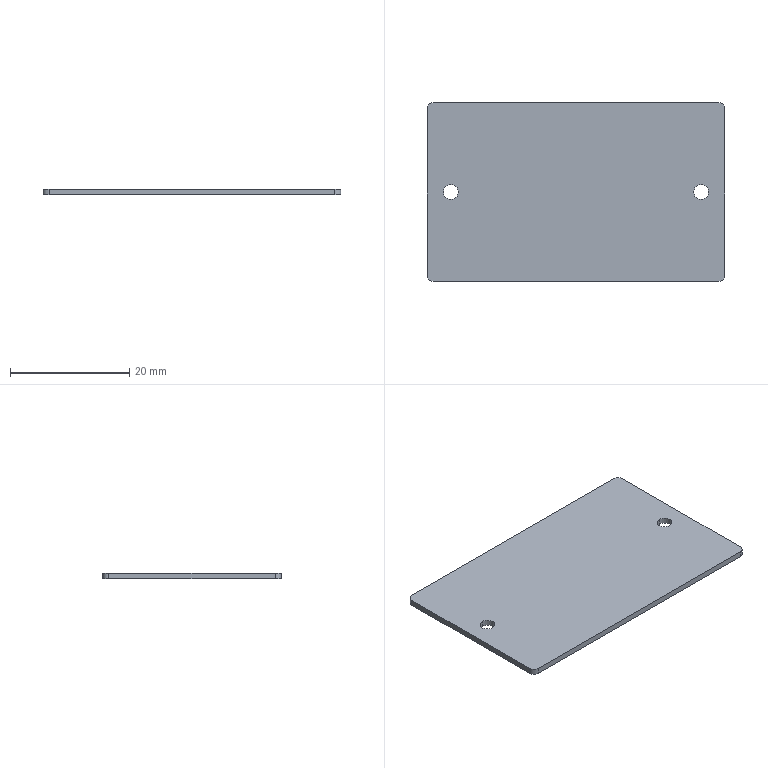Part | STEP file | Motor nameplate-Part-2 | 1 solid | 14 faces | box 50 x 30 x 1 mm | volume 1489 mm3 | cylinder 8 | plane 6 | commonest cylinder face diameters 2 x4 2.5 x4
STEP:
#1=CARTESIAN_POINT('',(0.,0.,0.));
#2=DIRECTION('',(0.,0.,1.));
#3=DIRECTION('',(1.,0.,0.));
#4=AXIS2_PLACEMENT_3D('',#1,#2,#3);
#5=CARTESIAN_POINT('',(-296.023,-35.783,51.8));
#6=VERTEX_POINT('',#5);
#7=CARTESIAN_POINT('',(-296.023,-35.783,50.8));
#8=VERTEX_POINT('',#7);
#9=CARTESIAN_POINT('',(-296.023,-35.783,51.8));
#10=DIRECTION('',(0.,0.,-1.));
#11=VECTOR('',#10,1.);
#12=LINE('',#9,#11);
#13=CARTESIAN_POINT('',(-296.023,-37.033,51.8));
#14=DIRECTION('',(0.,0.,-1.));
#15=DIRECTION('',(0.,1.,0.));
#16=AXIS2_PLACEMENT_3D('',#13,#14,#15);
#17=CYLINDRICAL_SURFACE('',#16,1.25);
#18=CARTESIAN_POINT('',(6.283,0.));
#19=DIRECTION('',(0.,1.));
#20=VECTOR('',#19,1.);
#21=LINE('',#18,#20);
#22=(GEOMETRIC_REPRESENTATION_CONTEXT(2)PARAMETRIC_REPRESENTATION_CONTEXT()REPRESENTATION_CONTEXT('',''));
#23=DEFINITIONAL_REPRESENTATION('',(#21),#22);
#24=PCURVE('',#17,#23);
#25=CARTESIAN_POINT('',(-296.023,-37.033,51.8));
#26=DIRECTION('',(0.,0.,-1.));
#27=DIRECTION('',(0.,1.,0.));
#28=AXIS2_PLACEMENT_3D('',#25,#26,#27);
#29=CYLINDRICAL_SURFACE('',#28,1.25);
#30=CARTESIAN_POINT('',(0.,0.));
#31=DIRECTION('',(0.,1.));
#32=VECTOR('',#31,1.);
#33=LINE('',#30,#32);
#34=(GEOMETRIC_REPRESENTATION_CONTEXT(2)PARAMETRIC_REPRESENTATION_CONTEXT()REPRESENTATION_CONTEXT('',''));
#35=DEFINITIONAL_REPRESENTATION('',(#33),#34);
#36=PCURVE('',#29,#35);
#37=SURFACE_CURVE('',#12,(#24,#36),.PCURVE_S1.);
#38=EDGE_CURVE('',#6,#8,#37,.T.);
#39=ORIENTED_EDGE('',*,*,#38,.T.);
#40=CARTESIAN_POINT('',(-296.023,-38.283,50.8));
#41=VERTEX_POINT('',#40);
#42=CARTESIAN_POINT('',(-296.023,-37.033,50.8));
#43=DIRECTION('',(0.,0.,1.));
#44=DIRECTION('',(0.,-1.,0.));
#45=AXIS2_PLACEMENT_3D('',#42,#43,#44);
#46=CIRCLE('',#45,1.25);
#47=CARTESIAN_POINT('',(9.425,1.));
#48=DIRECTION('',(-1.,0.));
#49=VECTOR('',#48,1.);
#50=LINE('',#47,#49);
#51=(GEOMETRIC_REPRESENTATION_CONTEXT(2)PARAMETRIC_REPRESENTATION_CONTEXT()REPRESENTATION_CONTEXT('',''));
#52=DEFINITIONAL_REPRESENTATION('',(#50),#51);
#53=PCURVE('',#17,#52);
#54=CARTESIAN_POINT('',(-275.023,-52.033,50.8));
#55=DIRECTION('',(0.,0.,-1.));
#56=DIRECTION('',(0.,1.,0.));
#57=AXIS2_PLACEMENT_3D('',#54,#55,#56);
#58=PLANE('',#57);
#59=CARTESIAN_POINT('',(13.75,-21.));
#60=CARTESIAN_POINT('',(13.75,-18.835));
#61=CARTESIAN_POINT('',(15.625,-19.917));
#62=CARTESIAN_POINT('',(17.5,-21.));
#63=CARTESIAN_POINT('',(15.625,-22.083));
#64=CARTESIAN_POINT('',(13.75,-23.165));
#65=CARTESIAN_POINT('',(13.75,-21.));
#66=(BOUNDED_CURVE()B_SPLINE_CURVE(2,(#59,#60,#61,#62,#63,#64,#65),.UNSPECIFIED.,.T.,.F.)B_SPLINE_CURVE_WITH_KNOTS((1,2,2,2,2,1),(-2.094,0.,2.094,4.189,6.283,8.378),.UNSPECIFIED.)CURVE()GEOMETRIC_REPRESENTATION_ITEM()RATIONAL_B_SPLINE_CURVE((1.,0.5,1.,0.5,1.,0.5,1.))REPRESENTATION_ITEM(''));
#67=(GEOMETRIC_REPRESENTATION_CONTEXT(2)PARAMETRIC_REPRESENTATION_CONTEXT()REPRESENTATION_CONTEXT('',''));
#68=DEFINITIONAL_REPRESENTATION('',(#66),#67);
#69=PCURVE('',#58,#68);
#70=SURFACE_CURVE('',#46,(#53,#69),.PCURVE_S1.);
#71=EDGE_CURVE('',#8,#41,#70,.T.);
#72=ORIENTED_EDGE('',*,*,#71,.T.);
#73=CARTESIAN_POINT('',(-296.023,-38.283,51.8));
#74=VERTEX_POINT('',#73);
#75=CARTESIAN_POINT('',(-296.023,-38.283,51.8));
#76=DIRECTION('',(0.,0.,-1.));
#77=VECTOR('',#76,1.);
#78=LINE('',#75,#77);
#79=CARTESIAN_POINT('',(3.142,0.));
#80=DIRECTION('',(0.,1.));
#81=VECTOR('',#80,1.);
#82=LINE('',#79,#81);
#83=(GEOMETRIC_REPRESENTATION_CONTEXT(2)PARAMETRIC_REPRESENTATION_CONTEXT()REPRESENTATION_CONTEXT('',''));
#84=DEFINITIONAL_REPRESENTATION('',(#82),#83);
#85=PCURVE('',#17,#84);
#86=CARTESIAN_POINT('',(3.142,0.));
#87=DIRECTION('',(0.,1.));
#88=VECTOR('',#87,1.);
#89=LINE('',#86,#88);
#90=(GEOMETRIC_REPRESENTATION_CONTEXT(2)PARAMETRIC_REPRESENTATION_CONTEXT()REPRESENTATION_CONTEXT('',''));
#91=DEFINITIONAL_REPRESENTATION('',(#89),#90);
#92=PCURVE('',#29,#91);
#93=SURFACE_CURVE('',#78,(#85,#92),.PCURVE_S1.);
#94=EDGE_CURVE('',#74,#41,#93,.T.);
#95=ORIENTED_EDGE('',*,*,#94,.F.);
#96=CARTESIAN_POINT('',(-296.023,-37.033,51.8));
#97=DIRECTION('',(0.,0.,-1.));
#98=DIRECTION('',(0.,1.,0.));
#99=AXIS2_PLACEMENT_3D('',#96,#97,#98);
#100=CIRCLE('',#99,1.25);
#101=CARTESIAN_POINT('',(0.,0.));
#102=DIRECTION('',(1.,0.));
#103=VECTOR('',#102,1.);
#104=LINE('',#101,#103);
#105=(GEOMETRIC_REPRESENTATION_CONTEXT(2)PARAMETRIC_REPRESENTATION_CONTEXT()REPRESENTATION_CONTEXT('',''));
#106=DEFINITIONAL_REPRESENTATION('',(#104),#105);
#107=PCURVE('',#17,#106);
#108=CARTESIAN_POINT('',(-275.023,-52.033,51.8));
#109=DIRECTION('',(0.,0.,1.));
#110=DIRECTION('',(0.,-1.,0.));
#111=AXIS2_PLACEMENT_3D('',#108,#109,#110);
#112=PLANE('',#111);
#113=CARTESIAN_POINT('',(-16.25,-21.));
#114=CARTESIAN_POINT('',(-16.25,-18.835));
#115=CARTESIAN_POINT('',(-14.375,-19.917));
#116=CARTESIAN_POINT('',(-12.5,-21.));
#117=CARTESIAN_POINT('',(-14.375,-22.083));
#118=CARTESIAN_POINT('',(-16.25,-23.165));
#119=CARTESIAN_POINT('',(-16.25,-21.));
#120=(BOUNDED_CURVE()B_SPLINE_CURVE(2,(#113,#114,#115,#116,#117,#118,#119),.UNSPECIFIED.,.T.,.F.)B_SPLINE_CURVE_WITH_KNOTS((1,2,2,2,2,1),(-2.094,0.,2.094,4.189,6.283,8.378),.UNSPECIFIED.)CURVE()GEOMETRIC_REPRESENTATION_ITEM()RATIONAL_B_SPLINE_CURVE((1.,0.5,1.,0.5,1.,0.5,1.))REPRESENTATION_ITEM(''));
#121=(GEOMETRIC_REPRESENTATION_CONTEXT(2)PARAMETRIC_REPRESENTATION_CONTEXT()REPRESENTATION_CONTEXT('',''));
#122=DEFINITIONAL_REPRESENTATION('',(#120),#121);
#123=PCURVE('',#112,#122);
#124=SURFACE_CURVE('',#100,(#107,#123),.PCURVE_S1.);
#125=EDGE_CURVE('',#74,#6,#124,.T.);
#126=ORIENTED_EDGE('',*,*,#125,.T.);
#127=EDGE_LOOP('',(#39,#72,#95,#126));
#128=FACE_BOUND('',#127,.F.);
#129=ADVANCED_FACE('',(#128),#17,.F.);
#130=CARTESIAN_POINT('',(-254.023,-35.783,51.8));
#131=VERTEX_POINT('',#130);
#132=CARTESIAN_POINT('',(-254.023,-35.783,50.8));
#133=VERTEX_POINT('',#132);
#134=CARTESIAN_POINT('',(-254.023,-35.783,51.8));
#135=DIRECTION('',(0.,0.,-1.));
#136=VECTOR('',#135,1.);
#137=LINE('',#134,#136);
#138=CARTESIAN_POINT('',(-254.023,-37.033,51.8));
#139=DIRECTION('',(0.,0.,-1.));
#140=DIRECTION('',(0.,1.,0.));
#141=AXIS2_PLACEMENT_3D('',#138,#139,#140);
#142=CYLINDRICAL_SURFACE('',#141,1.25);
#143=CARTESIAN_POINT('',(6.283,0.));
#144=DIRECTION('',(0.,1.));
#145=VECTOR('',#144,1.);
#146=LINE('',#143,#145);
#147=(GEOMETRIC_REPRESENTATION_CONTEXT(2)PARAMETRIC_REPRESENTATION_CONTEXT()REPRESENTATION_CONTEXT('',''));
#148=DEFINITIONAL_REPRESENTATION('',(#146),#147);
#149=PCURVE('',#142,#148);
#150=CARTESIAN_POINT('',(-254.023,-37.033,51.8));
#151=DIRECTION('',(0.,0.,-1.));
#152=DIRECTION('',(0.,1.,0.));
#153=AXIS2_PLACEMENT_3D('',#150,#151,#152);
#154=CYLINDRICAL_SURFACE('',#153,1.25);
#155=CARTESIAN_POINT('',(0.,0.));
#156=DIRECTION('',(0.,1.));
#157=VECTOR('',#156,1.);
#158=LINE('',#155,#157);
#159=(GEOMETRIC_REPRESENTATION_CONTEXT(2)PARAMETRIC_REPRESENTATION_CONTEXT()REPRESENTATION_CONTEXT('',''));
#160=DEFINITIONAL_REPRESENTATION('',(#158),#159);
#161=PCURVE('',#154,#160);
#162=SURFACE_CURVE('',#137,(#149,#161),.PCURVE_S1.);
#163=EDGE_CURVE('',#131,#133,#162,.T.);
#164=ORIENTED_EDGE('',*,*,#163,.T.);
#165=CARTESIAN_POINT('',(-254.023,-38.283,50.8));
#166=VERTEX_POINT('',#165);
#167=CARTESIAN_POINT('',(-254.023,-37.033,50.8));
#168=DIRECTION('',(0.,0.,1.));
#169=DIRECTION('',(0.,-1.,0.));
#170=AXIS2_PLACEMENT_3D('',#167,#168,#169);
#171=CIRCLE('',#170,1.25);
#172=CARTESIAN_POINT('',(9.425,1.));
#173=DIRECTION('',(-1.,0.));
#174=VECTOR('',#173,1.);
#175=LINE('',#172,#174);
#176=(GEOMETRIC_REPRESENTATION_CONTEXT(2)PARAMETRIC_REPRESENTATION_CONTEXT()REPRESENTATION_CONTEXT('',''));
#177=DEFINITIONAL_REPRESENTATION('',(#175),#176);
#178=PCURVE('',#142,#177);
#179=CARTESIAN_POINT('',(13.75,21.));
#180=CARTESIAN_POINT('',(13.75,23.165));
#181=CARTESIAN_POINT('',(15.625,22.083));
#182=CARTESIAN_POINT('',(17.5,21.));
#183=CARTESIAN_POINT('',(15.625,19.917));
#184=CARTESIAN_POINT('',(13.75,18.835));
#185=CARTESIAN_POINT('',(13.75,21.));
#186=(BOUNDED_CURVE()B_SPLINE_CURVE(2,(#179,#180,#181,#182,#183,#184,#185),.UNSPECIFIED.,.T.,.F.)B_SPLINE_CURVE_WITH_KNOTS((1,2,2,2,2,1),(-2.094,0.,2.094,4.189,6.283,8.378),.UNSPECIFIED.)CURVE()GEOMETRIC_REPRESENTATION_ITEM()RATIONAL_B_SPLINE_CURVE((1.,0.5,1.,0.5,1.,0.5,1.))REPRESENTATION_ITEM(''));
#187=(GEOMETRIC_REPRESENTATION_CONTEXT(2)PARAMETRIC_REPRESENTATION_CONTEXT()REPRESENTATION_CONTEXT('',''));
#188=DEFINITIONAL_REPRESENTATION('',(#186),#187);
#189=PCURVE('',#58,#188);
#190=SURFACE_CURVE('',#171,(#178,#189),.PCURVE_S1.);
#191=EDGE_CURVE('',#133,#166,#190,.T.);
#192=ORIENTED_EDGE('',*,*,#191,.T.);
#193=CARTESIAN_POINT('',(-254.023,-38.283,51.8));
#194=VERTEX_POINT('',#193);
#195=CARTESIAN_POINT('',(-254.023,-38.283,51.8));
#196=DIRECTION('',(0.,0.,-1.));
#197=VECTOR('',#196,1.);
#198=LINE('',#195,#197);
#199=CARTESIAN_POINT('',(3.142,0.));
#200=DIRECTION('',(0.,1.));
#201=VECTOR('',#200,1.);
#202=LINE('',#199,#201);
#203=(GEOMETRIC_REPRESENTATION_CONTEXT(2)PARAMETRIC_REPRESENTATION_CONTEXT()REPRESENTATION_CONTEXT('',''));
#204=DEFINITIONAL_REPRESENTATION('',(#202),#203);
#205=PCURVE('',#142,#204);
#206=CARTESIAN_POINT('',(3.142,0.));
#207=DIRECTION('',(0.,1.));
#208=VECTOR('',#207,1.);
#209=LINE('',#206,#208);
#210=(GEOMETRIC_REPRESENTATION_CONTEXT(2)PARAMETRIC_REPRESENTATION_CONTEXT()REPRESENTATION_CONTEXT('',''));
#211=DEFINITIONAL_REPRESENTATION('',(#209),#210);
#212=PCURVE('',#154,#211);
#213=SURFACE_CURVE('',#198,(#205,#212),.PCURVE_S1.);
#214=EDGE_CURVE('',#194,#166,#213,.T.);
#215=ORIENTED_EDGE('',*,*,#214,.F.);
#216=CARTESIAN_POINT('',(-254.023,-37.033,51.8));
#217=DIRECTION('',(0.,0.,-1.));
#218=DIRECTION('',(0.,1.,0.));
#219=AXIS2_PLACEMENT_3D('',#216,#217,#218);
#220=CIRCLE('',#219,1.25);
#221=CARTESIAN_POINT('',(0.,0.));
#222=DIRECTION('',(1.,0.));
#223=VECTOR('',#222,1.);
#224=LINE('',#221,#223);
#225=(GEOMETRIC_REPRESENTATION_CONTEXT(2)PARAMETRIC_REPRESENTATION_CONTEXT()REPRESENTATION_CONTEXT('',''));
#226=DEFINITIONAL_REPRESENTATION('',(#224),#225);
#227=PCURVE('',#142,#226);
#228=CARTESIAN_POINT('',(-16.25,21.));
#229=CARTESIAN_POINT('',(-16.25,23.165));
#230=CARTESIAN_POINT('',(-14.375,22.083));
#231=CARTESIAN_POINT('',(-12.5,21.));
#232=CARTESIAN_POINT('',(-14.375,19.917));
#233=CARTESIAN_POINT('',(-16.25,18.835));
#234=CARTESIAN_POINT('',(-16.25,21.));
#235=(BOUNDED_CURVE()B_SPLINE_CURVE(2,(#228,#229,#230,#231,#232,#233,#234),.UNSPECIFIED.,.T.,.F.)B_SPLINE_CURVE_WITH_KNOTS((1,2,2,2,2,1),(-2.094,0.,2.094,4.189,6.283,8.378),.UNSPECIFIED.)CURVE()GEOMETRIC_REPRESENTATION_ITEM()RATIONAL_B_SPLINE_CURVE((1.,0.5,1.,0.5,1.,0.5,1.))REPRESENTATION_ITEM(''));
#236=(GEOMETRIC_REPRESENTATION_CONTEXT(2)PARAMETRIC_REPRESENTATION_CONTEXT()REPRESENTATION_CONTEXT('',''));
#237=DEFINITIONAL_REPRESENTATION('',(#235),#236);
#238=PCURVE('',#112,#237);
#239=SURFACE_CURVE('',#220,(#227,#238),.PCURVE_S1.);
#240=EDGE_CURVE('',#194,#131,#239,.T.);
#241=ORIENTED_EDGE('',*,*,#240,.T.);
#242=EDGE_LOOP('',(#164,#192,#215,#241));
#243=FACE_BOUND('',#242,.F.);
#244=ADVANCED_FACE('',(#243),#142,.F.);
#245=CARTESIAN_POINT('',(-299.023,-22.033,50.8));
#246=VERTEX_POINT('',#245);
#247=CARTESIAN_POINT('',(-251.023,-22.033,50.8));
#248=VERTEX_POINT('',#247);
#249=CARTESIAN_POINT('',(-275.023,-22.033,50.8));
#250=DIRECTION('',(1.,0.,0.));
#251=VECTOR('',#250,1.);
#252=LINE('',#249,#251);
#253=CARTESIAN_POINT('',(-275.023,-22.033,51.3));
#254=DIRECTION('',(0.,1.,0.));
#255=DIRECTION('',(1.,0.,0.));
#256=AXIS2_PLACEMENT_3D('',#253,#254,#255);
#257=PLANE('',#256);
#258=CARTESIAN_POINT('',(0.,0.5));
#259=DIRECTION('',(1.,0.));
#260=VECTOR('',#259,1.);
#261=LINE('',#258,#260);
#262=(GEOMETRIC_REPRESENTATION_CONTEXT(2)PARAMETRIC_REPRESENTATION_CONTEXT()REPRESENTATION_CONTEXT('',''));
#263=DEFINITIONAL_REPRESENTATION('',(#261),#262);
#264=PCURVE('',#257,#263);
#265=CARTESIAN_POINT('',(30.,0.));
#266=DIRECTION('',(0.,1.));
#267=VECTOR('',#266,1.);
#268=LINE('',#265,#267);
#269=(GEOMETRIC_REPRESENTATION_CONTEXT(2)PARAMETRIC_REPRESENTATION_CONTEXT()REPRESENTATION_CONTEXT('',''));
#270=DEFINITIONAL_REPRESENTATION('',(#268),#269);
#271=PCURVE('',#58,#270);
#272=SURFACE_CURVE('',#252,(#264,#271),.PCURVE_S1.);
#273=EDGE_CURVE('',#246,#248,#272,.T.);
#274=ORIENTED_EDGE('',*,*,#273,.F.);
#275=CARTESIAN_POINT('',(-299.023,-22.033,51.8));
#276=VERTEX_POINT('',#275);
#277=CARTESIAN_POINT('',(-299.023,-22.033,51.3));
#278=DIRECTION('',(0.,0.,1.));
#279=VECTOR('',#278,1.);
#280=LINE('',#277,#279);
#281=CARTESIAN_POINT('',(-24.,0.));
#282=DIRECTION('',(0.,-1.));
#283=VECTOR('',#282,1.);
#284=LINE('',#281,#283);
#285=(GEOMETRIC_REPRESENTATION_CONTEXT(2)PARAMETRIC_REPRESENTATION_CONTEXT()REPRESENTATION_CONTEXT('',''));
#286=DEFINITIONAL_REPRESENTATION('',(#284),#285);
#287=PCURVE('',#257,#286);
#288=CARTESIAN_POINT('',(-299.023,-23.033,51.3));
#289=DIRECTION('',(0.,0.,-1.));
#290=DIRECTION('',(0.,1.,0.));
#291=AXIS2_PLACEMENT_3D('',#288,#289,#290);
#292=CYLINDRICAL_SURFACE('',#291,1.);
#293=CARTESIAN_POINT('',(6.283,0.));
#294=DIRECTION('',(0.,-1.));
#295=VECTOR('',#294,1.);
#296=LINE('',#293,#295);
#297=(GEOMETRIC_REPRESENTATION_CONTEXT(2)PARAMETRIC_REPRESENTATION_CONTEXT()REPRESENTATION_CONTEXT('',''));
#298=DEFINITIONAL_REPRESENTATION('',(#296),#297);
#299=PCURVE('',#292,#298);
#300=SURFACE_CURVE('',#280,(#287,#299),.PCURVE_S1.);
#301=EDGE_CURVE('',#246,#276,#300,.T.);
#302=ORIENTED_EDGE('',*,*,#301,.T.);
#303=CARTESIAN_POINT('',(-251.023,-22.033,51.8));
#304=VERTEX_POINT('',#303);
#305=CARTESIAN_POINT('',(-275.023,-22.033,51.8));
#306=DIRECTION('',(-1.,0.,0.));
#307=VECTOR('',#306,1.);
#308=LINE('',#305,#307);
#309=CARTESIAN_POINT('',(0.,-0.5));
#310=DIRECTION('',(-1.,0.));
#311=VECTOR('',#310,1.);
#312=LINE('',#309,#311);
#313=(GEOMETRIC_REPRESENTATION_CONTEXT(2)PARAMETRIC_REPRESENTATION_CONTEXT()REPRESENTATION_CONTEXT('',''));
#314=DEFINITIONAL_REPRESENTATION('',(#312),#313);
#315=PCURVE('',#257,#314);
#316=CARTESIAN_POINT('',(-30.,0.));
#317=DIRECTION('',(0.,-1.));
#318=VECTOR('',#317,1.);
#319=LINE('',#316,#318);
#320=(GEOMETRIC_REPRESENTATION_CONTEXT(2)PARAMETRIC_REPRESENTATION_CONTEXT()REPRESENTATION_CONTEXT('',''));
#321=DEFINITIONAL_REPRESENTATION('',(#319),#320);
#322=PCURVE('',#112,#321);
#323=SURFACE_CURVE('',#308,(#315,#322),.PCURVE_S1.);
#324=EDGE_CURVE('',#304,#276,#323,.T.);
#325=ORIENTED_EDGE('',*,*,#324,.F.);
#326=CARTESIAN_POINT('',(-251.023,-22.033,51.3));
#327=DIRECTION('',(0.,0.,-1.));
#328=VECTOR('',#327,1.);
#329=LINE('',#326,#328);
#330=CARTESIAN_POINT('',(24.,0.));
#331=DIRECTION('',(0.,1.));
#332=VECTOR('',#331,1.);
#333=LINE('',#330,#332);
#334=(GEOMETRIC_REPRESENTATION_CONTEXT(2)PARAMETRIC_REPRESENTATION_CONTEXT()REPRESENTATION_CONTEXT('',''));
#335=DEFINITIONAL_REPRESENTATION('',(#333),#334);
#336=PCURVE('',#257,#335);
#337=CARTESIAN_POINT('',(-251.023,-23.033,51.3));
#338=DIRECTION('',(0.,0.,1.));
#339=DIRECTION('',(0.,-1.,0.));
#340=AXIS2_PLACEMENT_3D('',#337,#338,#339);
#341=CYLINDRICAL_SURFACE('',#340,1.);
#342=CARTESIAN_POINT('',(3.142,0.));
#343=DIRECTION('',(0.,-1.));
#344=VECTOR('',#343,1.);
#345=LINE('',#342,#344);
#346=(GEOMETRIC_REPRESENTATION_CONTEXT(2)PARAMETRIC_REPRESENTATION_CONTEXT()REPRESENTATION_CONTEXT('',''));
#347=DEFINITIONAL_REPRESENTATION('',(#345),#346);
#348=PCURVE('',#341,#347);
#349=SURFACE_CURVE('',#329,(#336,#348),.PCURVE_S1.);
#350=EDGE_CURVE('',#304,#248,#349,.T.);
#351=ORIENTED_EDGE('',*,*,#350,.T.);
#352=EDGE_LOOP('',(#274,#302,#325,#351));
#353=FACE_BOUND('',#352,.T.);
#354=ADVANCED_FACE('',(#353),#257,.T.);
#355=CARTESIAN_POINT('',(-296.023,-37.033,51.8));
#356=DIRECTION('',(0.,0.,-1.));
#357=DIRECTION('',(0.,1.,0.));
#358=AXIS2_PLACEMENT_3D('',#355,#356,#357);
#359=CIRCLE('',#358,1.25);
#360=CARTESIAN_POINT('',(-16.25,-21.));
#361=CARTESIAN_POINT('',(-16.25,-18.835));
#362=CARTESIAN_POINT('',(-14.375,-19.917));
#363=CARTESIAN_POINT('',(-12.5,-21.));
#364=CARTESIAN_POINT('',(-14.375,-22.083));
#365=CARTESIAN_POINT('',(-16.25,-23.165));
#366=CARTESIAN_POINT('',(-16.25,-21.));
#367=(BOUNDED_CURVE()B_SPLINE_CURVE(2,(#360,#361,#362,#363,#364,#365,#366),.UNSPECIFIED.,.T.,.F.)B_SPLINE_CURVE_WITH_KNOTS((1,2,2,2,2,1),(-2.094,0.,2.094,4.189,6.283,8.378),.UNSPECIFIED.)CURVE()GEOMETRIC_REPRESENTATION_ITEM()RATIONAL_B_SPLINE_CURVE((1.,0.5,1.,0.5,1.,0.5,1.))REPRESENTATION_ITEM(''));
#368=(GEOMETRIC_REPRESENTATION_CONTEXT(2)PARAMETRIC_REPRESENTATION_CONTEXT()REPRESENTATION_CONTEXT('',''));
#369=DEFINITIONAL_REPRESENTATION('',(#367),#368);
#370=PCURVE('',#112,#369);
#371=CARTESIAN_POINT('',(0.,0.));
#372=DIRECTION('',(1.,0.));
#373=VECTOR('',#372,1.);
#374=LINE('',#371,#373);
#375=(GEOMETRIC_REPRESENTATION_CONTEXT(2)PARAMETRIC_REPRESENTATION_CONTEXT()REPRESENTATION_CONTEXT('',''));
#376=DEFINITIONAL_REPRESENTATION('',(#374),#375);
#377=PCURVE('',#29,#376);
#378=SURFACE_CURVE('',#359,(#370,#377),.PCURVE_S1.);
#379=EDGE_CURVE('',#6,#74,#378,.T.);
#380=ORIENTED_EDGE('',*,*,#379,.T.);
#381=ORIENTED_EDGE('',*,*,#125,.T.);
#382=EDGE_LOOP('',(#380,#381));
#383=FACE_BOUND('',#382,.T.);
#384=CARTESIAN_POINT('',(-254.023,-37.033,51.8));
#385=DIRECTION('',(0.,0.,-1.));
#386=DIRECTION('',(0.,1.,0.));
#387=AXIS2_PLACEMENT_3D('',#384,#385,#386);
#388=CIRCLE('',#387,1.25);
#389=CARTESIAN_POINT('',(-16.25,21.));
#390=CARTESIAN_POINT('',(-16.25,23.165));
#391=CARTESIAN_POINT('',(-14.375,22.083));
#392=CARTESIAN_POINT('',(-12.5,21.));
#393=CARTESIAN_POINT('',(-14.375,19.917));
#394=CARTESIAN_POINT('',(-16.25,18.835));
#395=CARTESIAN_POINT('',(-16.25,21.));
#396=(BOUNDED_CURVE()B_SPLINE_CURVE(2,(#389,#390,#391,#392,#393,#394,#395),.UNSPECIFIED.,.T.,.F.)B_SPLINE_CURVE_WITH_KNOTS((1,2,2,2,2,1),(-2.094,0.,2.094,4.189,6.283,8.378),.UNSPECIFIED.)CURVE()GEOMETRIC_REPRESENTATION_ITEM()RATIONAL_B_SPLINE_CURVE((1.,0.5,1.,0.5,1.,0.5,1.))REPRESENTATION_ITEM(''));
#397=(GEOMETRIC_REPRESENTATION_CONTEXT(2)PARAMETRIC_REPRESENTATION_CONTEXT()REPRESENTATION_CONTEXT('',''));
#398=DEFINITIONAL_REPRESENTATION('',(#396),#397);
#399=PCURVE('',#112,#398);
#400=CARTESIAN_POINT('',(0.,0.));
#401=DIRECTION('',(1.,0.));
#402=VECTOR('',#401,1.);
#403=LINE('',#400,#402);
#404=(GEOMETRIC_REPRESENTATION_CONTEXT(2)PARAMETRIC_REPRESENTATION_CONTEXT()REPRESENTATION_CONTEXT('',''));
#405=DEFINITIONAL_REPRESENTATION('',(#403),#404);
#406=PCURVE('',#154,#405);
#407=SURFACE_CURVE('',#388,(#399,#406),.PCURVE_S1.);
#408=EDGE_CURVE('',#131,#194,#407,.T.);
#409=ORIENTED_EDGE('',*,*,#408,.T.);
#410=ORIENTED_EDGE('',*,*,#240,.T.);
#411=EDGE_LOOP('',(#409,#410));
#412=FACE_BOUND('',#411,.T.);
#413=CARTESIAN_POINT('',(-300.023,-51.033,51.8));
#414=VERTEX_POINT('',#413);
#415=CARTESIAN_POINT('',(-300.023,-23.033,51.8));
#416=VERTEX_POINT('',#415);
#417=CARTESIAN_POINT('',(-300.023,-52.033,51.8));
#418=DIRECTION('',(0.,1.,0.));
#419=VECTOR('',#418,1.);
#420=LINE('',#417,#419);
#421=CARTESIAN_POINT('',(0.,-25.));
#422=DIRECTION('',(-1.,0.));
#423=VECTOR('',#422,1.);
#424=LINE('',#421,#423);
#425=(GEOMETRIC_REPRESENTATION_CONTEXT(2)PARAMETRIC_REPRESENTATION_CONTEXT()REPRESENTATION_CONTEXT('',''));
#426=DEFINITIONAL_REPRESENTATION('',(#424),#425);
#427=PCURVE('',#112,#426);
#428=CARTESIAN_POINT('',(-300.023,-52.033,51.3));
#429=DIRECTION('',(-1.,0.,0.));
#430=DIRECTION('',(0.,1.,0.));
#431=AXIS2_PLACEMENT_3D('',#428,#429,#430);
#432=PLANE('',#431);
#433=CARTESIAN_POINT('',(0.,-0.5));
#434=DIRECTION('',(1.,0.));
#435=VECTOR('',#434,1.);
#436=LINE('',#433,#435);
#437=(GEOMETRIC_REPRESENTATION_CONTEXT(2)PARAMETRIC_REPRESENTATION_CONTEXT()REPRESENTATION_CONTEXT('',''));
#438=DEFINITIONAL_REPRESENTATION('',(#436),#437);
#439=PCURVE('',#432,#438);
#440=SURFACE_CURVE('',#420,(#427,#439),.PCURVE_S1.);
#441=EDGE_CURVE('',#414,#416,#440,.T.);
#442=ORIENTED_EDGE('',*,*,#441,.F.);
#443=CARTESIAN_POINT('',(-299.023,-52.033,51.8));
#444=VERTEX_POINT('',#443);
#445=CARTESIAN_POINT('',(-299.023,-51.033,51.8));
#446=DIRECTION('',(0.,0.,1.));
#447=DIRECTION('',(0.,-1.,0.));
#448=AXIS2_PLACEMENT_3D('',#445,#446,#447);
#449=CIRCLE('',#448,1.);
#450=CARTESIAN_POINT('',(-1.,-24.));
#451=DIRECTION('',(1.,0.));
#452=AXIS2_PLACEMENT_2D('',#450,#451);
#453=CIRCLE('',#452,1.);
#454=(GEOMETRIC_REPRESENTATION_CONTEXT(2)PARAMETRIC_REPRESENTATION_CONTEXT()REPRESENTATION_CONTEXT('',''));
#455=DEFINITIONAL_REPRESENTATION('',(#453),#454);
#456=PCURVE('',#112,#455);
#457=CARTESIAN_POINT('',(-299.023,-51.033,51.3));
#458=DIRECTION('',(0.,0.,1.));
#459=DIRECTION('',(0.,-1.,0.));
#460=AXIS2_PLACEMENT_3D('',#457,#458,#459);
#461=CYLINDRICAL_SURFACE('',#460,1.);
#462=CARTESIAN_POINT('',(0.,0.5));
#463=DIRECTION('',(1.,0.));
#464=VECTOR('',#463,1.);
#465=LINE('',#462,#464);
#466=(GEOMETRIC_REPRESENTATION_CONTEXT(2)PARAMETRIC_REPRESENTATION_CONTEXT()REPRESENTATION_CONTEXT('',''));
#467=DEFINITIONAL_REPRESENTATION('',(#465),#466);
#468=PCURVE('',#461,#467);
#469=SURFACE_CURVE('',#449,(#456,#468),.PCURVE_S1.);
#470=EDGE_CURVE('',#414,#444,#469,.T.);
#471=ORIENTED_EDGE('',*,*,#470,.T.);
#472=CARTESIAN_POINT('',(-251.023,-52.033,51.8));
#473=VERTEX_POINT('',#472);
#474=CARTESIAN_POINT('',(-275.023,-52.033,51.8));
#475=DIRECTION('',(1.,0.,0.));
#476=VECTOR('',#475,1.);
#477=LINE('',#474,#476);
#478=CARTESIAN_POINT('',(0.,0.));
#479=DIRECTION('',(0.,1.));
#480=VECTOR('',#479,1.);
#481=LINE('',#478,#480);
#482=(GEOMETRIC_REPRESENTATION_CONTEXT(2)PARAMETRIC_REPRESENTATION_CONTEXT()REPRESENTATION_CONTEXT('',''));
#483=DEFINITIONAL_REPRESENTATION('',(#481),#482);
#484=PCURVE('',#112,#483);
#485=CARTESIAN_POINT('',(-275.023,-52.033,51.3));
#486=DIRECTION('',(0.,-1.,0.));
#487=DIRECTION('',(-1.,0.,0.));
#488=AXIS2_PLACEMENT_3D('',#485,#486,#487);
#489=PLANE('',#488);
#490=CARTESIAN_POINT('',(0.,-0.5));
#491=DIRECTION('',(-1.,0.));
#492=VECTOR('',#491,1.);
#493=LINE('',#490,#492);
#494=(GEOMETRIC_REPRESENTATION_CONTEXT(2)PARAMETRIC_REPRESENTATION_CONTEXT()REPRESENTATION_CONTEXT('',''));
#495=DEFINITIONAL_REPRESENTATION('',(#493),#494);
#496=PCURVE('',#489,#495);
#497=SURFACE_CURVE('',#477,(#484,#496),.PCURVE_S1.);
#498=EDGE_CURVE('',#444,#473,#497,.T.);
#499=ORIENTED_EDGE('',*,*,#498,.T.);
#500=CARTESIAN_POINT('',(-250.023,-51.033,51.8));
#501=VERTEX_POINT('',#500);
#502=CARTESIAN_POINT('',(-251.023,-51.033,51.8));
#503=DIRECTION('',(0.,0.,1.));
#504=DIRECTION('',(0.,-1.,0.));
#505=AXIS2_PLACEMENT_3D('',#502,#503,#504);
#506=CIRCLE('',#505,1.);
#507=CARTESIAN_POINT('',(-1.,24.));
#508=DIRECTION('',(1.,0.));
#509=AXIS2_PLACEMENT_2D('',#507,#508);
#510=CIRCLE('',#509,1.);
#511=(GEOMETRIC_REPRESENTATION_CONTEXT(2)PARAMETRIC_REPRESENTATION_CONTEXT()REPRESENTATION_CONTEXT('',''));
#512=DEFINITIONAL_REPRESENTATION('',(#510),#511);
#513=PCURVE('',#112,#512);
#514=CARTESIAN_POINT('',(-251.023,-51.033,51.3));
#515=DIRECTION('',(0.,0.,-1.));
#516=DIRECTION('',(0.,1.,0.));
#517=AXIS2_PLACEMENT_3D('',#514,#515,#516);
#518=CYLINDRICAL_SURFACE('',#517,1.);
#519=CARTESIAN_POINT('',(3.142,-0.5));
#520=DIRECTION('',(-1.,0.));
#521=VECTOR('',#520,1.);
#522=LINE('',#519,#521);
#523=(GEOMETRIC_REPRESENTATION_CONTEXT(2)PARAMETRIC_REPRESENTATION_CONTEXT()REPRESENTATION_CONTEXT('',''));
#524=DEFINITIONAL_REPRESENTATION('',(#522),#523);
#525=PCURVE('',#518,#524);
#526=SURFACE_CURVE('',#506,(#513,#525),.PCURVE_S1.);
#527=EDGE_CURVE('',#473,#501,#526,.T.);
#528=ORIENTED_EDGE('',*,*,#527,.T.);
#529=CARTESIAN_POINT('',(-250.023,-23.033,51.8));
#530=VERTEX_POINT('',#529);
#531=CARTESIAN_POINT('',(-250.023,-52.033,51.8));
#532=DIRECTION('',(0.,1.,0.));
#533=VECTOR('',#532,1.);
#534=LINE('',#531,#533);
#535=CARTESIAN_POINT('',(0.,25.));
#536=DIRECTION('',(-1.,0.));
#537=VECTOR('',#536,1.);
#538=LINE('',#535,#537);
#539=(GEOMETRIC_REPRESENTATION_CONTEXT(2)PARAMETRIC_REPRESENTATION_CONTEXT()REPRESENTATION_CONTEXT('',''));
#540=DEFINITIONAL_REPRESENTATION('',(#538),#539);
#541=PCURVE('',#112,#540);
#542=CARTESIAN_POINT('',(-250.023,-52.033,51.3));
#543=DIRECTION('',(1.,0.,0.));
#544=DIRECTION('',(0.,-1.,0.));
#545=AXIS2_PLACEMENT_3D('',#542,#543,#544);
#546=PLANE('',#545);
#547=CARTESIAN_POINT('',(0.,-0.5));
#548=DIRECTION('',(-1.,0.));
#549=VECTOR('',#548,1.);
#550=LINE('',#547,#549);
#551=(GEOMETRIC_REPRESENTATION_CONTEXT(2)PARAMETRIC_REPRESENTATION_CONTEXT()REPRESENTATION_CONTEXT('',''));
#552=DEFINITIONAL_REPRESENTATION('',(#550),#551);
#553=PCURVE('',#546,#552);
#554=SURFACE_CURVE('',#534,(#541,#553),.PCURVE_S1.);
#555=EDGE_CURVE('',#501,#530,#554,.T.);
#556=ORIENTED_EDGE('',*,*,#555,.T.);
#557=CARTESIAN_POINT('',(-251.023,-23.033,51.8));
#558=DIRECTION('',(0.,0.,1.));
#559=DIRECTION('',(0.,-1.,0.));
#560=AXIS2_PLACEMENT_3D('',#557,#558,#559);
#561=CIRCLE('',#560,1.);
#562=CARTESIAN_POINT('',(-29.,24.));
#563=DIRECTION('',(1.,0.));
#564=AXIS2_PLACEMENT_2D('',#562,#563);
#565=CIRCLE('',#564,1.);
#566=(GEOMETRIC_REPRESENTATION_CONTEXT(2)PARAMETRIC_REPRESENTATION_CONTEXT()REPRESENTATION_CONTEXT('',''));
#567=DEFINITIONAL_REPRESENTATION('',(#565),#566);
#568=PCURVE('',#112,#567);
#569=CARTESIAN_POINT('',(0.,0.5));
#570=DIRECTION('',(1.,0.));
#571=VECTOR('',#570,1.);
#572=LINE('',#569,#571);
#573=(GEOMETRIC_REPRESENTATION_CONTEXT(2)PARAMETRIC_REPRESENTATION_CONTEXT()REPRESENTATION_CONTEXT('',''));
#574=DEFINITIONAL_REPRESENTATION('',(#572),#573);
#575=PCURVE('',#341,#574);
#576=SURFACE_CURVE('',#561,(#568,#575),.PCURVE_S1.);
#577=EDGE_CURVE('',#530,#304,#576,.T.);
#578=ORIENTED_EDGE('',*,*,#577,.T.);
#579=ORIENTED_EDGE('',*,*,#324,.T.);
#580=CARTESIAN_POINT('',(-299.023,-23.033,51.8));
#581=DIRECTION('',(0.,0.,1.));
#582=DIRECTION('',(0.,-1.,0.));
#583=AXIS2_PLACEMENT_3D('',#580,#581,#582);
#584=CIRCLE('',#583,1.);
#585=CARTESIAN_POINT('',(-29.,-24.));
#586=DIRECTION('',(1.,0.));
#587=AXIS2_PLACEMENT_2D('',#585,#586);
#588=CIRCLE('',#587,1.);
#589=(GEOMETRIC_REPRESENTATION_CONTEXT(2)PARAMETRIC_REPRESENTATION_CONTEXT()REPRESENTATION_CONTEXT('',''));
#590=DEFINITIONAL_REPRESENTATION('',(#588),#589);
#591=PCURVE('',#112,#590);
#592=CARTESIAN_POINT('',(9.425,-0.5));
#593=DIRECTION('',(-1.,0.));
#594=VECTOR('',#593,1.);
#595=LINE('',#592,#594);
#596=(GEOMETRIC_REPRESENTATION_CONTEXT(2)PARAMETRIC_REPRESENTATION_CONTEXT()REPRESENTATION_CONTEXT('',''));
#597=DEFINITIONAL_REPRESENTATION('',(#595),#596);
#598=PCURVE('',#292,#597);
#599=SURFACE_CURVE('',#584,(#591,#598),.PCURVE_S1.);
#600=EDGE_CURVE('',#276,#416,#599,.T.);
#601=ORIENTED_EDGE('',*,*,#600,.T.);
#602=EDGE_LOOP('',(#442,#471,#499,#528,#556,#578,#579,#601));
#603=FACE_BOUND('',#602,.T.);
#604=ADVANCED_FACE('',(#383,#412,#603),#112,.T.);
#605=CARTESIAN_POINT('',(-300.023,-51.033,50.8));
#606=VERTEX_POINT('',#605);
#607=CARTESIAN_POINT('',(-300.023,-23.033,50.8));
#608=VERTEX_POINT('',#607);
#609=CARTESIAN_POINT('',(-300.023,-52.033,50.8));
#610=DIRECTION('',(0.,1.,0.));
#611=VECTOR('',#610,1.);
#612=LINE('',#609,#611);
#613=CARTESIAN_POINT('',(0.,0.5));
#614=DIRECTION('',(1.,0.));
#615=VECTOR('',#614,1.);
#616=LINE('',#613,#615);
#617=(GEOMETRIC_REPRESENTATION_CONTEXT(2)PARAMETRIC_REPRESENTATION_CONTEXT()REPRESENTATION_CONTEXT('',''));
#618=DEFINITIONAL_REPRESENTATION('',(#616),#617);
#619=PCURVE('',#432,#618);
#620=CARTESIAN_POINT('',(0.,-25.));
#621=DIRECTION('',(1.,0.));
#622=VECTOR('',#621,1.);
#623=LINE('',#620,#622);
#624=(GEOMETRIC_REPRESENTATION_CONTEXT(2)PARAMETRIC_REPRESENTATION_CONTEXT()REPRESENTATION_CONTEXT('',''));
#625=DEFINITIONAL_REPRESENTATION('',(#623),#624);
#626=PCURVE('',#58,#625);
#627=SURFACE_CURVE('',#612,(#619,#626),.PCURVE_S1.);
#628=EDGE_CURVE('',#606,#608,#627,.T.);
#629=ORIENTED_EDGE('',*,*,#628,.F.);
#630=CARTESIAN_POINT('',(-300.023,-51.033,51.3));
#631=DIRECTION('',(0.,0.,1.));
#632=VECTOR('',#631,1.);
#633=LINE('',#630,#632);
#634=CARTESIAN_POINT('',(1.,0.));
#635=DIRECTION('',(0.,-1.));
#636=VECTOR('',#635,1.);
#637=LINE('',#634,#636);
#638=(GEOMETRIC_REPRESENTATION_CONTEXT(2)PARAMETRIC_REPRESENTATION_CONTEXT()REPRESENTATION_CONTEXT('',''));
#639=DEFINITIONAL_REPRESENTATION('',(#637),#638);
#640=PCURVE('',#432,#639);
#641=CARTESIAN_POINT('',(4.712,0.));
#642=DIRECTION('',(0.,1.));
#643=VECTOR('',#642,1.);
#644=LINE('',#641,#643);
#645=(GEOMETRIC_REPRESENTATION_CONTEXT(2)PARAMETRIC_REPRESENTATION_CONTEXT()REPRESENTATION_CONTEXT('',''));
#646=DEFINITIONAL_REPRESENTATION('',(#644),#645);
#647=PCURVE('',#461,#646);
#648=SURFACE_CURVE('',#633,(#640,#647),.PCURVE_S1.);
#649=EDGE_CURVE('',#606,#414,#648,.T.);
#650=ORIENTED_EDGE('',*,*,#649,.T.);
#651=ORIENTED_EDGE('',*,*,#441,.T.);
#652=CARTESIAN_POINT('',(-300.023,-23.033,51.3));
#653=DIRECTION('',(0.,0.,-1.));
#654=VECTOR('',#653,1.);
#655=LINE('',#652,#654);
#656=CARTESIAN_POINT('',(29.,0.));
#657=DIRECTION('',(0.,1.));
#658=VECTOR('',#657,1.);
#659=LINE('',#656,#658);
#660=(GEOMETRIC_REPRESENTATION_CONTEXT(2)PARAMETRIC_REPRESENTATION_CONTEXT()REPRESENTATION_CONTEXT('',''));
#661=DEFINITIONAL_REPRESENTATION('',(#659),#660);
#662=PCURVE('',#432,#661);
#663=CARTESIAN_POINT('',(4.712,0.));
#664=DIRECTION('',(0.,1.));
#665=VECTOR('',#664,1.);
#666=LINE('',#663,#665);
#667=(GEOMETRIC_REPRESENTATION_CONTEXT(2)PARAMETRIC_REPRESENTATION_CONTEXT()REPRESENTATION_CONTEXT('',''));
#668=DEFINITIONAL_REPRESENTATION('',(#666),#667);
#669=PCURVE('',#292,#668);
#670=SURFACE_CURVE('',#655,(#662,#669),.PCURVE_S1.);
#671=EDGE_CURVE('',#416,#608,#670,.T.);
#672=ORIENTED_EDGE('',*,*,#671,.T.);
#673=EDGE_LOOP('',(#629,#650,#651,#672));
#674=FACE_BOUND('',#673,.T.);
#675=ADVANCED_FACE('',(#674),#432,.T.);
#676=ORIENTED_EDGE('',*,*,#71,.T.);
#677=CARTESIAN_POINT('',(-296.023,-37.033,50.8));
#678=DIRECTION('',(0.,0.,1.));
#679=DIRECTION('',(0.,-1.,0.));
#680=AXIS2_PLACEMENT_3D('',#677,#678,#679);
#681=CIRCLE('',#680,1.25);
#682=CARTESIAN_POINT('',(13.75,-21.));
#683=CARTESIAN_POINT('',(13.75,-18.835));
#684=CARTESIAN_POINT('',(15.625,-19.917));
#685=CARTESIAN_POINT('',(17.5,-21.));
#686=CARTESIAN_POINT('',(15.625,-22.083));
#687=CARTESIAN_POINT('',(13.75,-23.165));
#688=CARTESIAN_POINT('',(13.75,-21.));
#689=(BOUNDED_CURVE()B_SPLINE_CURVE(2,(#682,#683,#684,#685,#686,#687,#688),.UNSPECIFIED.,.T.,.F.)B_SPLINE_CURVE_WITH_KNOTS((1,2,2,2,2,1),(-2.094,0.,2.094,4.189,6.283,8.378),.UNSPECIFIED.)CURVE()GEOMETRIC_REPRESENTATION_ITEM()RATIONAL_B_SPLINE_CURVE((1.,0.5,1.,0.5,1.,0.5,1.))REPRESENTATION_ITEM(''));
#690=(GEOMETRIC_REPRESENTATION_CONTEXT(2)PARAMETRIC_REPRESENTATION_CONTEXT()REPRESENTATION_CONTEXT('',''));
#691=DEFINITIONAL_REPRESENTATION('',(#689),#690);
#692=PCURVE('',#58,#691);
#693=CARTESIAN_POINT('',(3.142,1.));
#694=DIRECTION('',(-1.,0.));
#695=VECTOR('',#694,1.);
#696=LINE('',#693,#695);
#697=(GEOMETRIC_REPRESENTATION_CONTEXT(2)PARAMETRIC_REPRESENTATION_CONTEXT()REPRESENTATION_CONTEXT('',''));
#698=DEFINITIONAL_REPRESENTATION('',(#696),#697);
#699=PCURVE('',#29,#698);
#700=SURFACE_CURVE('',#681,(#692,#699),.PCURVE_S1.);
#701=EDGE_CURVE('',#41,#8,#700,.T.);
#702=ORIENTED_EDGE('',*,*,#701,.T.);
#703=EDGE_LOOP('',(#676,#702));
#704=FACE_BOUND('',#703,.T.);
#705=ORIENTED_EDGE('',*,*,#191,.T.);
#706=CARTESIAN_POINT('',(-254.023,-37.033,50.8));
#707=DIRECTION('',(0.,0.,1.));
#708=DIRECTION('',(0.,-1.,0.));
#709=AXIS2_PLACEMENT_3D('',#706,#707,#708);
#710=CIRCLE('',#709,1.25);
#711=CARTESIAN_POINT('',(13.75,21.));
#712=CARTESIAN_POINT('',(13.75,23.165));
#713=CARTESIAN_POINT('',(15.625,22.083));
#714=CARTESIAN_POINT('',(17.5,21.));
#715=CARTESIAN_POINT('',(15.625,19.917));
#716=CARTESIAN_POINT('',(13.75,18.835));
#717=CARTESIAN_POINT('',(13.75,21.));
#718=(BOUNDED_CURVE()B_SPLINE_CURVE(2,(#711,#712,#713,#714,#715,#716,#717),.UNSPECIFIED.,.T.,.F.)B_SPLINE_CURVE_WITH_KNOTS((1,2,2,2,2,1),(-2.094,0.,2.094,4.189,6.283,8.378),.UNSPECIFIED.)CURVE()GEOMETRIC_REPRESENTATION_ITEM()RATIONAL_B_SPLINE_CURVE((1.,0.5,1.,0.5,1.,0.5,1.))REPRESENTATION_ITEM(''));
#719=(GEOMETRIC_REPRESENTATION_CONTEXT(2)PARAMETRIC_REPRESENTATION_CONTEXT()REPRESENTATION_CONTEXT('',''));
#720=DEFINITIONAL_REPRESENTATION('',(#718),#719);
#721=PCURVE('',#58,#720);
#722=CARTESIAN_POINT('',(3.142,1.));
#723=DIRECTION('',(-1.,0.));
#724=VECTOR('',#723,1.);
#725=LINE('',#722,#724);
#726=(GEOMETRIC_REPRESENTATION_CONTEXT(2)PARAMETRIC_REPRESENTATION_CONTEXT()REPRESENTATION_CONTEXT('',''));
#727=DEFINITIONAL_REPRESENTATION('',(#725),#726);
#728=PCURVE('',#154,#727);
#729=SURFACE_CURVE('',#710,(#721,#728),.PCURVE_S1.);
#730=EDGE_CURVE('',#166,#133,#729,.T.);
#731=ORIENTED_EDGE('',*,*,#730,.T.);
#732=EDGE_LOOP('',(#705,#731));
#733=FACE_BOUND('',#732,.T.);
#734=CARTESIAN_POINT('',(-251.023,-52.033,50.8));
#735=VERTEX_POINT('',#734);
#736=CARTESIAN_POINT('',(-299.023,-52.033,50.8));
#737=VERTEX_POINT('',#736);
#738=CARTESIAN_POINT('',(-275.023,-52.033,50.8));
#739=DIRECTION('',(-1.,0.,0.));
#740=VECTOR('',#739,1.);
#741=LINE('',#738,#740);
#742=CARTESIAN_POINT('',(0.,0.));
#743=DIRECTION('',(0.,-1.));
#744=VECTOR('',#743,1.);
#745=LINE('',#742,#744);
#746=(GEOMETRIC_REPRESENTATION_CONTEXT(2)PARAMETRIC_REPRESENTATION_CONTEXT()REPRESENTATION_CONTEXT('',''));
#747=DEFINITIONAL_REPRESENTATION('',(#745),#746);
#748=PCURVE('',#58,#747);
#749=CARTESIAN_POINT('',(0.,0.5));
#750=DIRECTION('',(1.,0.));
#751=VECTOR('',#750,1.);
#752=LINE('',#749,#751);
#753=(GEOMETRIC_REPRESENTATION_CONTEXT(2)PARAMETRIC_REPRESENTATION_CONTEXT()REPRESENTATION_CONTEXT('',''));
#754=DEFINITIONAL_REPRESENTATION('',(#752),#753);
#755=PCURVE('',#489,#754);
#756=SURFACE_CURVE('',#741,(#748,#755),.PCURVE_S1.);
#757=EDGE_CURVE('',#735,#737,#756,.T.);
#758=ORIENTED_EDGE('',*,*,#757,.T.);
#759=CARTESIAN_POINT('',(-299.023,-51.033,50.8));
#760=DIRECTION('',(0.,0.,-1.));
#761=DIRECTION('',(0.,1.,0.));
#762=AXIS2_PLACEMENT_3D('',#759,#760,#761);
#763=CIRCLE('',#762,1.);
#764=CARTESIAN_POINT('',(1.,-24.));
#765=DIRECTION('',(1.,0.));
#766=AXIS2_PLACEMENT_2D('',#764,#765);
#767=CIRCLE('',#766,1.);
#768=(GEOMETRIC_REPRESENTATION_CONTEXT(2)PARAMETRIC_REPRESENTATION_CONTEXT()REPRESENTATION_CONTEXT('',''));
#769=DEFINITIONAL_REPRESENTATION('',(#767),#768);
#770=PCURVE('',#58,#769);
#771=CARTESIAN_POINT('',(9.425,-0.5));
#772=DIRECTION('',(-1.,0.));
#773=VECTOR('',#772,1.);
#774=LINE('',#771,#773);
#775=(GEOMETRIC_REPRESENTATION_CONTEXT(2)PARAMETRIC_REPRESENTATION_CONTEXT()REPRESENTATION_CONTEXT('',''));
#776=DEFINITIONAL_REPRESENTATION('',(#774),#775);
#777=PCURVE('',#461,#776);
#778=SURFACE_CURVE('',#763,(#770,#777),.PCURVE_S1.);
#779=EDGE_CURVE('',#737,#606,#778,.T.);
#780=ORIENTED_EDGE('',*,*,#779,.T.);
#781=ORIENTED_EDGE('',*,*,#628,.T.);
#782=CARTESIAN_POINT('',(-299.023,-23.033,50.8));
#783=DIRECTION('',(0.,0.,-1.));
#784=DIRECTION('',(0.,1.,0.));
#785=AXIS2_PLACEMENT_3D('',#782,#783,#784);
#786=CIRCLE('',#785,1.);
#787=CARTESIAN_POINT('',(29.,-24.));
#788=DIRECTION('',(1.,0.));
#789=AXIS2_PLACEMENT_2D('',#787,#788);
#790=CIRCLE('',#789,1.);
#791=(GEOMETRIC_REPRESENTATION_CONTEXT(2)PARAMETRIC_REPRESENTATION_CONTEXT()REPRESENTATION_CONTEXT('',''));
#792=DEFINITIONAL_REPRESENTATION('',(#790),#791);
#793=PCURVE('',#58,#792);
#794=CARTESIAN_POINT('',(0.,0.5));
#795=DIRECTION('',(1.,0.));
#796=VECTOR('',#795,1.);
#797=LINE('',#794,#796);
#798=(GEOMETRIC_REPRESENTATION_CONTEXT(2)PARAMETRIC_REPRESENTATION_CONTEXT()REPRESENTATION_CONTEXT('',''));
#799=DEFINITIONAL_REPRESENTATION('',(#797),#798);
#800=PCURVE('',#292,#799);
#801=SURFACE_CURVE('',#786,(#793,#800),.PCURVE_S1.);
#802=EDGE_CURVE('',#608,#246,#801,.T.);
#803=ORIENTED_EDGE('',*,*,#802,.T.);
#804=ORIENTED_EDGE('',*,*,#273,.T.);
#805=CARTESIAN_POINT('',(-250.023,-23.033,50.8));
#806=VERTEX_POINT('',#805);
#807=CARTESIAN_POINT('',(-251.023,-23.033,50.8));
#808=DIRECTION('',(0.,0.,-1.));
#809=DIRECTION('',(0.,1.,0.));
#810=AXIS2_PLACEMENT_3D('',#807,#808,#809);
#811=CIRCLE('',#810,1.);
#812=CARTESIAN_POINT('',(29.,24.));
#813=DIRECTION('',(1.,0.));
#814=AXIS2_PLACEMENT_2D('',#812,#813);
#815=CIRCLE('',#814,1.);
#816=(GEOMETRIC_REPRESENTATION_CONTEXT(2)PARAMETRIC_REPRESENTATION_CONTEXT()REPRESENTATION_CONTEXT('',''));
#817=DEFINITIONAL_REPRESENTATION('',(#815),#816);
#818=PCURVE('',#58,#817);
#819=CARTESIAN_POINT('',(3.142,-0.5));
#820=DIRECTION('',(-1.,0.));
#821=VECTOR('',#820,1.);
#822=LINE('',#819,#821);
#823=(GEOMETRIC_REPRESENTATION_CONTEXT(2)PARAMETRIC_REPRESENTATION_CONTEXT()REPRESENTATION_CONTEXT('',''));
#824=DEFINITIONAL_REPRESENTATION('',(#822),#823);
#825=PCURVE('',#341,#824);
#826=SURFACE_CURVE('',#811,(#818,#825),.PCURVE_S1.);
#827=EDGE_CURVE('',#248,#806,#826,.T.);
#828=ORIENTED_EDGE('',*,*,#827,.T.);
#829=CARTESIAN_POINT('',(-250.023,-51.033,50.8));
#830=VERTEX_POINT('',#829);
#831=CARTESIAN_POINT('',(-250.023,-52.033,50.8));
#832=DIRECTION('',(0.,1.,0.));
#833=VECTOR('',#832,1.);
#834=LINE('',#831,#833);
#835=CARTESIAN_POINT('',(0.,25.));
#836=DIRECTION('',(1.,0.));
#837=VECTOR('',#836,1.);
#838=LINE('',#835,#837);
#839=(GEOMETRIC_REPRESENTATION_CONTEXT(2)PARAMETRIC_REPRESENTATION_CONTEXT()REPRESENTATION_CONTEXT('',''));
#840=DEFINITIONAL_REPRESENTATION('',(#838),#839);
#841=PCURVE('',#58,#840);
#842=CARTESIAN_POINT('',(0.,0.5));
#843=DIRECTION('',(-1.,0.));
#844=VECTOR('',#843,1.);
#845=LINE('',#842,#844);
#846=(GEOMETRIC_REPRESENTATION_CONTEXT(2)PARAMETRIC_REPRESENTATION_CONTEXT()REPRESENTATION_CONTEXT('',''));
#847=DEFINITIONAL_REPRESENTATION('',(#845),#846);
#848=PCURVE('',#546,#847);
#849=SURFACE_CURVE('',#834,(#841,#848),.PCURVE_S1.);
#850=EDGE_CURVE('',#830,#806,#849,.T.);
#851=ORIENTED_EDGE('',*,*,#850,.F.);
#852=CARTESIAN_POINT('',(-251.023,-51.033,50.8));
#853=DIRECTION('',(0.,0.,-1.));
#854=DIRECTION('',(0.,1.,0.));
#855=AXIS2_PLACEMENT_3D('',#852,#853,#854);
#856=CIRCLE('',#855,1.);
#857=CARTESIAN_POINT('',(1.,24.));
#858=DIRECTION('',(1.,0.));
#859=AXIS2_PLACEMENT_2D('',#857,#858);
#860=CIRCLE('',#859,1.);
#861=(GEOMETRIC_REPRESENTATION_CONTEXT(2)PARAMETRIC_REPRESENTATION_CONTEXT()REPRESENTATION_CONTEXT('',''));
#862=DEFINITIONAL_REPRESENTATION('',(#860),#861);
#863=PCURVE('',#58,#862);
#864=CARTESIAN_POINT('',(0.,0.5));
#865=DIRECTION('',(1.,0.));
#866=VECTOR('',#865,1.);
#867=LINE('',#864,#866);
#868=(GEOMETRIC_REPRESENTATION_CONTEXT(2)PARAMETRIC_REPRESENTATION_CONTEXT()REPRESENTATION_CONTEXT('',''));
#869=DEFINITIONAL_REPRESENTATION('',(#867),#868);
#870=PCURVE('',#518,#869);
#871=SURFACE_CURVE('',#856,(#863,#870),.PCURVE_S1.);
#872=EDGE_CURVE('',#830,#735,#871,.T.);
#873=ORIENTED_EDGE('',*,*,#872,.T.);
#874=EDGE_LOOP('',(#758,#780,#781,#803,#804,#828,#851,#873));
#875=FACE_BOUND('',#874,.T.);
#876=ADVANCED_FACE('',(#704,#733,#875),#58,.T.);
#877=ORIENTED_EDGE('',*,*,#498,.F.);
#878=CARTESIAN_POINT('',(-299.023,-52.033,51.3));
#879=DIRECTION('',(0.,0.,-1.));
#880=VECTOR('',#879,1.);
#881=LINE('',#878,#880);
#882=CARTESIAN_POINT('',(24.,0.));
#883=DIRECTION('',(0.,1.));
#884=VECTOR('',#883,1.);
#885=LINE('',#882,#884);
#886=(GEOMETRIC_REPRESENTATION_CONTEXT(2)PARAMETRIC_REPRESENTATION_CONTEXT()REPRESENTATION_CONTEXT('',''));
#887=DEFINITIONAL_REPRESENTATION('',(#885),#886);
#888=PCURVE('',#489,#887);
#889=CARTESIAN_POINT('',(6.283,0.));
#890=DIRECTION('',(0.,-1.));
#891=VECTOR('',#890,1.);
#892=LINE('',#889,#891);
#893=(GEOMETRIC_REPRESENTATION_CONTEXT(2)PARAMETRIC_REPRESENTATION_CONTEXT()REPRESENTATION_CONTEXT('',''));
#894=DEFINITIONAL_REPRESENTATION('',(#892),#893);
#895=PCURVE('',#461,#894);
#896=SURFACE_CURVE('',#881,(#888,#895),.PCURVE_S1.);
#897=EDGE_CURVE('',#444,#737,#896,.T.);
#898=ORIENTED_EDGE('',*,*,#897,.T.);
#899=ORIENTED_EDGE('',*,*,#757,.F.);
#900=CARTESIAN_POINT('',(-251.023,-52.033,51.3));
#901=DIRECTION('',(0.,0.,1.));
#902=VECTOR('',#901,1.);
#903=LINE('',#900,#902);
#904=CARTESIAN_POINT('',(-24.,0.));
#905=DIRECTION('',(0.,-1.));
#906=VECTOR('',#905,1.);
#907=LINE('',#904,#906);
#908=(GEOMETRIC_REPRESENTATION_CONTEXT(2)PARAMETRIC_REPRESENTATION_CONTEXT()REPRESENTATION_CONTEXT('',''));
#909=DEFINITIONAL_REPRESENTATION('',(#907),#908);
#910=PCURVE('',#489,#909);
#911=CARTESIAN_POINT('',(3.142,0.));
#912=DIRECTION('',(0.,-1.));
#913=VECTOR('',#912,1.);
#914=LINE('',#911,#913);
#915=(GEOMETRIC_REPRESENTATION_CONTEXT(2)PARAMETRIC_REPRESENTATION_CONTEXT()REPRESENTATION_CONTEXT('',''));
#916=DEFINITIONAL_REPRESENTATION('',(#914),#915);
#917=PCURVE('',#518,#916);
#918=SURFACE_CURVE('',#903,(#910,#917),.PCURVE_S1.);
#919=EDGE_CURVE('',#735,#473,#918,.T.);
#920=ORIENTED_EDGE('',*,*,#919,.T.);
#921=EDGE_LOOP('',(#877,#898,#899,#920));
#922=FACE_BOUND('',#921,.T.);
#923=ADVANCED_FACE('',(#922),#489,.T.);
#924=ORIENTED_EDGE('',*,*,#555,.F.);
#925=CARTESIAN_POINT('',(-250.023,-51.033,51.3));
#926=DIRECTION('',(0.,0.,-1.));
#927=VECTOR('',#926,1.);
#928=LINE('',#925,#927);
#929=CARTESIAN_POINT('',(-1.,0.));
#930=DIRECTION('',(0.,1.));
#931=VECTOR('',#930,1.);
#932=LINE('',#929,#931);
#933=(GEOMETRIC_REPRESENTATION_CONTEXT(2)PARAMETRIC_REPRESENTATION_CONTEXT()REPRESENTATION_CONTEXT('',''));
#934=DEFINITIONAL_REPRESENTATION('',(#932),#933);
#935=PCURVE('',#546,#934);
#936=CARTESIAN_POINT('',(1.571,0.));
#937=DIRECTION('',(0.,1.));
#938=VECTOR('',#937,1.);
#939=LINE('',#936,#938);
#940=(GEOMETRIC_REPRESENTATION_CONTEXT(2)PARAMETRIC_REPRESENTATION_CONTEXT()REPRESENTATION_CONTEXT('',''));
#941=DEFINITIONAL_REPRESENTATION('',(#939),#940);
#942=PCURVE('',#518,#941);
#943=SURFACE_CURVE('',#928,(#935,#942),.PCURVE_S1.);
#944=EDGE_CURVE('',#501,#830,#943,.T.);
#945=ORIENTED_EDGE('',*,*,#944,.T.);
#946=ORIENTED_EDGE('',*,*,#850,.T.);
#947=CARTESIAN_POINT('',(-250.023,-23.033,51.3));
#948=DIRECTION('',(0.,0.,1.));
#949=VECTOR('',#948,1.);
#950=LINE('',#947,#949);
#951=CARTESIAN_POINT('',(-29.,0.));
#952=DIRECTION('',(0.,-1.));
#953=VECTOR('',#952,1.);
#954=LINE('',#951,#953);
#955=(GEOMETRIC_REPRESENTATION_CONTEXT(2)PARAMETRIC_REPRESENTATION_CONTEXT()REPRESENTATION_CONTEXT('',''));
#956=DEFINITIONAL_REPRESENTATION('',(#954),#955);
#957=PCURVE('',#546,#956);
#958=CARTESIAN_POINT('',(1.571,0.));
#959=DIRECTION('',(0.,1.));
#960=VECTOR('',#959,1.);
#961=LINE('',#958,#960);
#962=(GEOMETRIC_REPRESENTATION_CONTEXT(2)PARAMETRIC_REPRESENTATION_CONTEXT()REPRESENTATION_CONTEXT('',''));
#963=DEFINITIONAL_REPRESENTATION('',(#961),#962);
#964=PCURVE('',#341,#963);
#965=SURFACE_CURVE('',#950,(#957,#964),.PCURVE_S1.);
#966=EDGE_CURVE('',#806,#530,#965,.T.);
#967=ORIENTED_EDGE('',*,*,#966,.T.);
#968=EDGE_LOOP('',(#924,#945,#946,#967));
#969=FACE_BOUND('',#968,.T.);
#970=ADVANCED_FACE('',(#969),#546,.T.);
#971=ORIENTED_EDGE('',*,*,#827,.F.);
#972=ORIENTED_EDGE('',*,*,#350,.F.);
#973=ORIENTED_EDGE('',*,*,#577,.F.);
#974=ORIENTED_EDGE('',*,*,#966,.F.);
#975=EDGE_LOOP('',(#971,#972,#973,#974));
#976=FACE_BOUND('',#975,.T.);
#977=ADVANCED_FACE('',(#976),#341,.T.);
#978=ORIENTED_EDGE('',*,*,#527,.F.);
#979=ORIENTED_EDGE('',*,*,#919,.F.);
#980=ORIENTED_EDGE('',*,*,#872,.F.);
#981=ORIENTED_EDGE('',*,*,#944,.F.);
#982=EDGE_LOOP('',(#978,#979,#980,#981));
#983=FACE_BOUND('',#982,.T.);
#984=ADVANCED_FACE('',(#983),#518,.T.);
#985=ORIENTED_EDGE('',*,*,#600,.F.);
#986=ORIENTED_EDGE('',*,*,#301,.F.);
#987=ORIENTED_EDGE('',*,*,#802,.F.);
#988=ORIENTED_EDGE('',*,*,#671,.F.);
#989=EDGE_LOOP('',(#985,#986,#987,#988));
#990=FACE_BOUND('',#989,.T.);
#991=ADVANCED_FACE('',(#990),#292,.T.);
#992=ORIENTED_EDGE('',*,*,#779,.F.);
#993=ORIENTED_EDGE('',*,*,#897,.F.);
#994=ORIENTED_EDGE('',*,*,#470,.F.);
#995=ORIENTED_EDGE('',*,*,#649,.F.);
#996=EDGE_LOOP('',(#992,#993,#994,#995));
#997=FACE_BOUND('',#996,.T.);
#998=ADVANCED_FACE('',(#997),#461,.T.);
#999=ORIENTED_EDGE('',*,*,#730,.T.);
#1000=ORIENTED_EDGE('',*,*,#163,.F.);
#1001=ORIENTED_EDGE('',*,*,#408,.T.);
#1002=ORIENTED_EDGE('',*,*,#214,.T.);
#1003=EDGE_LOOP('',(#999,#1000,#1001,#1002));
#1004=FACE_BOUND('',#1003,.F.);
#1005=ADVANCED_FACE('',(#1004),#154,.F.);
#1006=ORIENTED_EDGE('',*,*,#701,.T.);
#1007=ORIENTED_EDGE('',*,*,#38,.F.);
#1008=ORIENTED_EDGE('',*,*,#379,.T.);
#1009=ORIENTED_EDGE('',*,*,#94,.T.);
#1010=EDGE_LOOP('',(#1006,#1007,#1008,#1009));
#1011=FACE_BOUND('',#1010,.F.);
#1012=ADVANCED_FACE('',(#1011),#29,.F.);
#1013=CLOSED_SHELL('',(#129,#244,#354,#604,#675,#876,#923,#970,#977,#984,#991,#998,#1005,#1012));
#1014=MANIFOLD_SOLID_BREP('',#1013);
#1015=(LENGTH_UNIT()NAMED_UNIT(*)SI_UNIT(.MILLI.,.METRE.));
#1016=UNCERTAINTY_MEASURE_WITH_UNIT(LENGTH_MEASURE(0.0000001),#1015,'','');
#1017=(NAMED_UNIT(*)PLANE_ANGLE_UNIT()SI_UNIT($,.RADIAN.));
#1018=(NAMED_UNIT(*)SI_UNIT($,.STERADIAN.)SOLID_ANGLE_UNIT());
#1019=(GEOMETRIC_REPRESENTATION_CONTEXT(3)GLOBAL_UNCERTAINTY_ASSIGNED_CONTEXT((#1016))GLOBAL_UNIT_ASSIGNED_CONTEXT((#1015,#1017,#1018))REPRESENTATION_CONTEXT('',''));
#1020=ADVANCED_BREP_SHAPE_REPRESENTATION('',(#4,#1014),#1019);